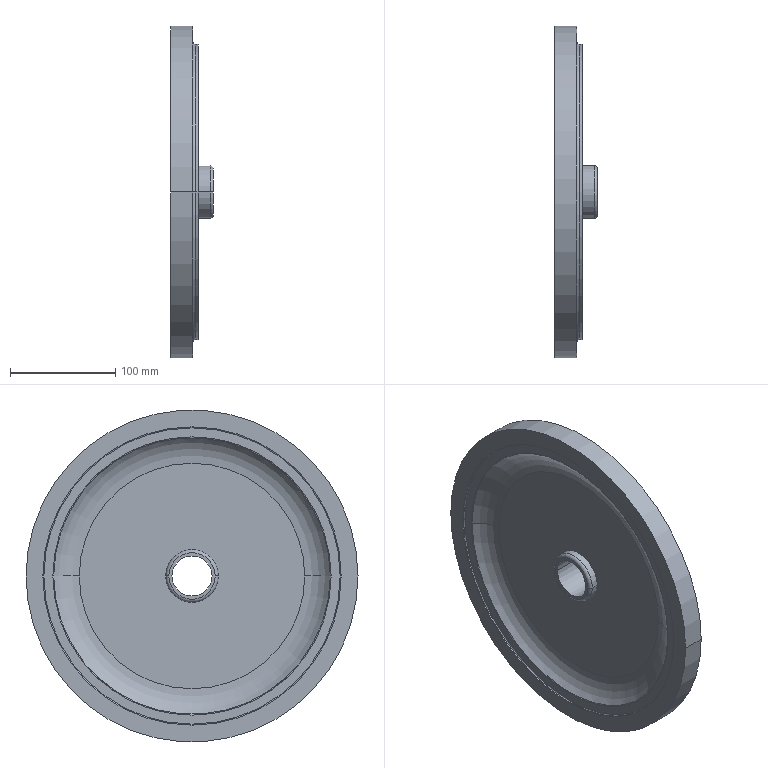Part | SolidWorks | features Revolution 1 | 1 solid | 31 faces | box 40.5 x 315 x 315 mm | volume 1243951 mm3 | torus 12 | cylinder 12 | plane 7 | commonest cylinder face diameters 50 x4 38 x2 280 x2 283 x2 315 x2
STEP:
#1=CARTESIAN_POINT('',(-149.425,-131.204,0.));
#2=VERTEX_POINT('',#1);
#3=CARTESIAN_POINT('',(-149.425,131.204,0.));
#4=VERTEX_POINT('',#3);
#5=CARTESIAN_POINT('',(-149.425,0.,0.));
#6=DIRECTION('',(1.,0.,0.));
#7=DIRECTION('',(0.,1.,0.));
#8=AXIS2_PLACEMENT_3D('',#5,#6,#7);
#9=CIRCLE('',#8,131.204);
#10=EDGE_CURVE('',#2,#4,#9,.T.);
#11=ORIENTED_EDGE('',*,*,#10,.F.);
#12=CARTESIAN_POINT('',(-137.8,-107.,0.));
#13=VERTEX_POINT('',#12);
#14=CARTESIAN_POINT('',(-168.81,-107.,0.));
#15=DIRECTION('',(0.,0.,1.));
#16=DIRECTION('',(0.,-1.,0.));
#17=AXIS2_PLACEMENT_3D('',#14,#15,#16);
#18=CIRCLE('',#17,31.01);
#19=EDGE_CURVE('',#2,#13,#18,.T.);
#20=ORIENTED_EDGE('',*,*,#19,.T.);
#21=CARTESIAN_POINT('',(-137.8,107.,0.));
#22=VERTEX_POINT('',#21);
#23=CARTESIAN_POINT('',(-137.8,0.,0.));
#24=DIRECTION('',(1.,0.,0.));
#25=DIRECTION('',(0.,1.,0.));
#26=AXIS2_PLACEMENT_3D('',#23,#24,#25);
#27=CIRCLE('',#26,107.);
#28=EDGE_CURVE('',#13,#22,#27,.T.);
#29=ORIENTED_EDGE('',*,*,#28,.T.);
#30=CARTESIAN_POINT('',(-168.81,107.,0.));
#31=DIRECTION('',(0.,0.,-1.));
#32=DIRECTION('',(-1.,0.,0.));
#33=AXIS2_PLACEMENT_3D('',#30,#31,#32);
#34=CIRCLE('',#33,31.01);
#35=EDGE_CURVE('',#4,#22,#34,.T.);
#36=ORIENTED_EDGE('',*,*,#35,.F.);
#37=EDGE_LOOP('',(#11,#20,#29,#36));
#38=FACE_OUTER_BOUND('',#37,.T.);
#39=CARTESIAN_POINT('',(-168.81,0.,0.));
#40=DIRECTION('',(1.,0.,0.));
#41=DIRECTION('',(0.,1.,0.));
#42=AXIS2_PLACEMENT_3D('',#39,#40,#41);
#43=TOROIDAL_SURFACE('',#42,107.,31.01);
#44=ADVANCED_FACE('',(#38),#43,.F.);
#45=CARTESIAN_POINT('',(-149.425,0.,0.));
#46=DIRECTION('',(1.,0.,0.));
#47=DIRECTION('',(0.,1.,0.));
#48=AXIS2_PLACEMENT_3D('',#45,#46,#47);
#49=CIRCLE('',#48,131.204);
#50=EDGE_CURVE('',#4,#2,#49,.T.);
#51=ORIENTED_EDGE('',*,*,#50,.T.);
#52=CARTESIAN_POINT('',(-149.8,-131.985,0.));
#53=VERTEX_POINT('',#52);
#54=CARTESIAN_POINT('',(-148.8,-131.985,0.));
#55=DIRECTION('',(0.,0.,1.));
#56=DIRECTION('',(0.,-1.,0.));
#57=AXIS2_PLACEMENT_3D('',#54,#55,#56);
#58=CIRCLE('',#57,1.);
#59=EDGE_CURVE('',#2,#53,#58,.T.);
#60=ORIENTED_EDGE('',*,*,#59,.T.);
#61=CARTESIAN_POINT('',(-149.8,131.985,0.));
#62=VERTEX_POINT('',#61);
#63=CARTESIAN_POINT('',(-149.8,0.,0.));
#64=DIRECTION('',(1.,0.,0.));
#65=DIRECTION('',(0.,1.,0.));
#66=AXIS2_PLACEMENT_3D('',#63,#64,#65);
#67=CIRCLE('',#66,131.985);
#68=EDGE_CURVE('',#62,#53,#67,.T.);
#69=ORIENTED_EDGE('',*,*,#68,.F.);
#70=CARTESIAN_POINT('',(-148.8,131.985,0.));
#71=DIRECTION('',(0.,0.,-1.));
#72=DIRECTION('',(-1.,0.,0.));
#73=AXIS2_PLACEMENT_3D('',#70,#71,#72);
#74=CIRCLE('',#73,1.);
#75=EDGE_CURVE('',#4,#62,#74,.T.);
#76=ORIENTED_EDGE('',*,*,#75,.F.);
#77=EDGE_LOOP('',(#51,#60,#69,#76));
#78=FACE_OUTER_BOUND('',#77,.T.);
#79=CARTESIAN_POINT('',(-148.8,0.,0.));
#80=DIRECTION('',(1.,0.,0.));
#81=DIRECTION('',(0.,1.,0.));
#82=AXIS2_PLACEMENT_3D('',#79,#80,#81);
#83=TOROIDAL_SURFACE('',#82,131.985,1.);
#84=ADVANCED_FACE('',(#78),#83,.T.);
#85=CARTESIAN_POINT('',(-150.8,-141.5,0.));
#86=VERTEX_POINT('',#85);
#87=CARTESIAN_POINT('',(-150.8,141.5,0.));
#88=VERTEX_POINT('',#87);
#89=CARTESIAN_POINT('',(-150.8,0.,0.));
#90=DIRECTION('',(1.,0.,0.));
#91=DIRECTION('',(0.,1.,0.));
#92=AXIS2_PLACEMENT_3D('',#89,#90,#91);
#93=CIRCLE('',#92,141.5);
#94=EDGE_CURVE('',#86,#88,#93,.T.);
#95=ORIENTED_EDGE('',*,*,#94,.F.);
#96=CARTESIAN_POINT('',(-149.8,-140.5,0.));
#97=VERTEX_POINT('',#96);
#98=CARTESIAN_POINT('',(-150.8,-140.5,0.));
#99=DIRECTION('',(0.,0.,1.));
#100=DIRECTION('',(0.,-1.,0.));
#101=AXIS2_PLACEMENT_3D('',#98,#99,#100);
#102=CIRCLE('',#101,1.);
#103=EDGE_CURVE('',#86,#97,#102,.T.);
#104=ORIENTED_EDGE('',*,*,#103,.T.);
#105=CARTESIAN_POINT('',(-149.8,140.5,0.));
#106=VERTEX_POINT('',#105);
#107=CARTESIAN_POINT('',(-149.8,0.,0.));
#108=DIRECTION('',(1.,0.,0.));
#109=DIRECTION('',(0.,1.,0.));
#110=AXIS2_PLACEMENT_3D('',#107,#108,#109);
#111=CIRCLE('',#110,140.5);
#112=EDGE_CURVE('',#97,#106,#111,.T.);
#113=ORIENTED_EDGE('',*,*,#112,.T.);
#114=CARTESIAN_POINT('',(-150.8,140.5,0.));
#115=DIRECTION('',(0.,0.,-1.));
#116=DIRECTION('',(-1.,0.,0.));
#117=AXIS2_PLACEMENT_3D('',#114,#115,#116);
#118=CIRCLE('',#117,1.);
#119=EDGE_CURVE('',#88,#106,#118,.T.);
#120=ORIENTED_EDGE('',*,*,#119,.F.);
#121=EDGE_LOOP('',(#95,#104,#113,#120));
#122=FACE_OUTER_BOUND('',#121,.T.);
#123=CARTESIAN_POINT('',(-150.8,0.,0.));
#124=DIRECTION('',(1.,0.,0.));
#125=DIRECTION('',(0.,1.,0.));
#126=AXIS2_PLACEMENT_3D('',#123,#124,#125);
#127=TOROIDAL_SURFACE('',#126,140.5,1.);
#128=ADVANCED_FACE('',(#122),#127,.F.);
#129=CARTESIAN_POINT('',(-151.8,-141.5,0.));
#130=VERTEX_POINT('',#129);
#131=CARTESIAN_POINT('',(-151.8,141.5,0.));
#132=VERTEX_POINT('',#131);
#133=CARTESIAN_POINT('',(-151.8,0.,0.));
#134=DIRECTION('',(1.,0.,0.));
#135=DIRECTION('',(0.,1.,0.));
#136=AXIS2_PLACEMENT_3D('',#133,#134,#135);
#137=CIRCLE('',#136,141.5);
#138=EDGE_CURVE('',#130,#132,#137,.T.);
#139=ORIENTED_EDGE('',*,*,#138,.F.);
#140=CARTESIAN_POINT('',(-55.,-141.5,0.));
#141=DIRECTION('',(1.,0.,0.));
#142=VECTOR('',#141,1000.);
#143=LINE('',#140,#142);
#144=EDGE_CURVE('',#130,#86,#143,.T.);
#145=ORIENTED_EDGE('',*,*,#144,.T.);
#146=ORIENTED_EDGE('',*,*,#94,.T.);
#147=CARTESIAN_POINT('',(-55.,141.5,0.));
#148=DIRECTION('',(1.,0.,0.));
#149=VECTOR('',#148,1000.);
#150=LINE('',#147,#149);
#151=EDGE_CURVE('',#132,#88,#150,.T.);
#152=ORIENTED_EDGE('',*,*,#151,.F.);
#153=EDGE_LOOP('',(#139,#145,#146,#152));
#154=FACE_OUTER_BOUND('',#153,.T.);
#155=CARTESIAN_POINT('',(-55.,0.,0.));
#156=DIRECTION('',(1.,0.,0.));
#157=DIRECTION('',(0.,1.,0.));
#158=AXIS2_PLACEMENT_3D('',#155,#156,#157);
#159=CYLINDRICAL_SURFACE('',#158,141.5);
#160=ADVANCED_FACE('',(#154),#159,.F.);
#161=CARTESIAN_POINT('',(-151.8,157.5,0.));
#162=VERTEX_POINT('',#161);
#163=CARTESIAN_POINT('',(-151.8,-157.5,0.));
#164=VERTEX_POINT('',#163);
#165=CARTESIAN_POINT('',(-151.8,0.,0.));
#166=DIRECTION('',(1.,0.,0.));
#167=DIRECTION('',(0.,1.,0.));
#168=AXIS2_PLACEMENT_3D('',#165,#166,#167);
#169=CIRCLE('',#168,157.5);
#170=EDGE_CURVE('',#162,#164,#169,.T.);
#171=ORIENTED_EDGE('',*,*,#170,.T.);
#172=CARTESIAN_POINT('',(-130.8,-157.5,0.));
#173=VERTEX_POINT('',#172);
#174=CARTESIAN_POINT('',(-55.,-157.5,0.));
#175=DIRECTION('',(1.,0.,0.));
#176=VECTOR('',#175,1000.);
#177=LINE('',#174,#176);
#178=EDGE_CURVE('',#164,#173,#177,.T.);
#179=ORIENTED_EDGE('',*,*,#178,.T.);
#180=CARTESIAN_POINT('',(-130.8,157.5,0.));
#181=VERTEX_POINT('',#180);
#182=CARTESIAN_POINT('',(-130.8,0.,0.));
#183=DIRECTION('',(1.,0.,0.));
#184=DIRECTION('',(0.,1.,0.));
#185=AXIS2_PLACEMENT_3D('',#182,#183,#184);
#186=CIRCLE('',#185,157.5);
#187=EDGE_CURVE('',#181,#173,#186,.T.);
#188=ORIENTED_EDGE('',*,*,#187,.F.);
#189=CARTESIAN_POINT('',(-55.,157.5,0.));
#190=DIRECTION('',(1.,0.,0.));
#191=VECTOR('',#190,1000.);
#192=LINE('',#189,#191);
#193=EDGE_CURVE('',#162,#181,#192,.T.);
#194=ORIENTED_EDGE('',*,*,#193,.F.);
#195=EDGE_LOOP('',(#171,#179,#188,#194));
#196=FACE_OUTER_BOUND('',#195,.T.);
#197=CARTESIAN_POINT('',(-55.,0.,0.));
#198=DIRECTION('',(1.,0.,0.));
#199=DIRECTION('',(0.,1.,0.));
#200=AXIS2_PLACEMENT_3D('',#197,#198,#199);
#201=CYLINDRICAL_SURFACE('',#200,157.5);
#202=ADVANCED_FACE('',(#196),#201,.T.);
#203=CARTESIAN_POINT('',(-128.3,-140.,0.));
#204=VERTEX_POINT('',#203);
#205=CARTESIAN_POINT('',(-128.3,140.,0.));
#206=VERTEX_POINT('',#205);
#207=CARTESIAN_POINT('',(-128.3,0.,0.));
#208=DIRECTION('',(1.,0.,0.));
#209=DIRECTION('',(0.,1.,0.));
#210=AXIS2_PLACEMENT_3D('',#207,#208,#209);
#211=CIRCLE('',#210,140.);
#212=EDGE_CURVE('',#204,#206,#211,.T.);
#213=ORIENTED_EDGE('',*,*,#212,.F.);
#214=CARTESIAN_POINT('',(-130.8,-142.5,0.));
#215=VERTEX_POINT('',#214);
#216=CARTESIAN_POINT('',(-128.3,-142.5,0.));
#217=DIRECTION('',(0.,0.,1.));
#218=DIRECTION('',(0.,-1.,0.));
#219=AXIS2_PLACEMENT_3D('',#216,#217,#218);
#220=CIRCLE('',#219,2.5);
#221=EDGE_CURVE('',#204,#215,#220,.T.);
#222=ORIENTED_EDGE('',*,*,#221,.T.);
#223=CARTESIAN_POINT('',(-130.8,142.5,0.));
#224=VERTEX_POINT('',#223);
#225=CARTESIAN_POINT('',(-130.8,0.,0.));
#226=DIRECTION('',(1.,0.,0.));
#227=DIRECTION('',(0.,1.,0.));
#228=AXIS2_PLACEMENT_3D('',#225,#226,#227);
#229=CIRCLE('',#228,142.5);
#230=EDGE_CURVE('',#215,#224,#229,.T.);
#231=ORIENTED_EDGE('',*,*,#230,.T.);
#232=CARTESIAN_POINT('',(-128.3,142.5,0.));
#233=DIRECTION('',(0.,0.,-1.));
#234=DIRECTION('',(-1.,0.,0.));
#235=AXIS2_PLACEMENT_3D('',#232,#233,#234);
#236=CIRCLE('',#235,2.5);
#237=EDGE_CURVE('',#206,#224,#236,.T.);
#238=ORIENTED_EDGE('',*,*,#237,.F.);
#239=EDGE_LOOP('',(#213,#222,#231,#238));
#240=FACE_OUTER_BOUND('',#239,.T.);
#241=CARTESIAN_POINT('',(-128.3,0.,0.));
#242=DIRECTION('',(1.,0.,0.));
#243=DIRECTION('',(0.,1.,0.));
#244=AXIS2_PLACEMENT_3D('',#241,#242,#243);
#245=TOROIDAL_SURFACE('',#244,142.5,2.5);
#246=ADVANCED_FACE('',(#240),#245,.F.);
#247=CARTESIAN_POINT('',(-128.3,0.,0.));
#248=DIRECTION('',(1.,0.,0.));
#249=DIRECTION('',(0.,1.,0.));
#250=AXIS2_PLACEMENT_3D('',#247,#248,#249);
#251=CIRCLE('',#250,140.);
#252=EDGE_CURVE('',#206,#204,#251,.T.);
#253=ORIENTED_EDGE('',*,*,#252,.T.);
#254=CARTESIAN_POINT('',(-125.8,-140.,0.));
#255=VERTEX_POINT('',#254);
#256=CARTESIAN_POINT('',(-55.,-140.,0.));
#257=DIRECTION('',(1.,0.,0.));
#258=VECTOR('',#257,1000.);
#259=LINE('',#256,#258);
#260=EDGE_CURVE('',#204,#255,#259,.T.);
#261=ORIENTED_EDGE('',*,*,#260,.T.);
#262=CARTESIAN_POINT('',(-125.8,140.,0.));
#263=VERTEX_POINT('',#262);
#264=CARTESIAN_POINT('',(-125.8,0.,0.));
#265=DIRECTION('',(1.,0.,0.));
#266=DIRECTION('',(0.,1.,0.));
#267=AXIS2_PLACEMENT_3D('',#264,#265,#266);
#268=CIRCLE('',#267,140.);
#269=EDGE_CURVE('',#263,#255,#268,.T.);
#270=ORIENTED_EDGE('',*,*,#269,.F.);
#271=CARTESIAN_POINT('',(-55.,140.,0.));
#272=DIRECTION('',(1.,0.,0.));
#273=VECTOR('',#272,1000.);
#274=LINE('',#271,#273);
#275=EDGE_CURVE('',#206,#263,#274,.T.);
#276=ORIENTED_EDGE('',*,*,#275,.F.);
#277=EDGE_LOOP('',(#253,#261,#270,#276));
#278=FACE_OUTER_BOUND('',#277,.T.);
#279=CARTESIAN_POINT('',(-55.,0.,0.));
#280=DIRECTION('',(1.,0.,0.));
#281=DIRECTION('',(0.,1.,0.));
#282=AXIS2_PLACEMENT_3D('',#279,#280,#281);
#283=CYLINDRICAL_SURFACE('',#282,140.);
#284=ADVANCED_FACE('',(#278),#283,.T.);
#285=CARTESIAN_POINT('',(-125.8,25.,0.));
#286=VERTEX_POINT('',#285);
#287=CARTESIAN_POINT('',(-125.8,-25.,0.));
#288=VERTEX_POINT('',#287);
#289=CARTESIAN_POINT('',(-125.8,0.,0.));
#290=DIRECTION('',(1.,0.,0.));
#291=DIRECTION('',(0.,1.,0.));
#292=AXIS2_PLACEMENT_3D('',#289,#290,#291);
#293=CIRCLE('',#292,25.);
#294=EDGE_CURVE('',#286,#288,#293,.T.);
#295=ORIENTED_EDGE('',*,*,#294,.T.);
#296=CARTESIAN_POINT('',(-114.3,-25.,0.));
#297=VERTEX_POINT('',#296);
#298=CARTESIAN_POINT('',(-55.,-25.,0.));
#299=DIRECTION('',(1.,0.,0.));
#300=VECTOR('',#299,1000.);
#301=LINE('',#298,#300);
#302=EDGE_CURVE('',#288,#297,#301,.T.);
#303=ORIENTED_EDGE('',*,*,#302,.T.);
#304=CARTESIAN_POINT('',(-114.3,25.,0.));
#305=VERTEX_POINT('',#304);
#306=CARTESIAN_POINT('',(-114.3,0.,0.));
#307=DIRECTION('',(1.,0.,0.));
#308=DIRECTION('',(0.,1.,0.));
#309=AXIS2_PLACEMENT_3D('',#306,#307,#308);
#310=CIRCLE('',#309,25.);
#311=EDGE_CURVE('',#305,#297,#310,.T.);
#312=ORIENTED_EDGE('',*,*,#311,.F.);
#313=CARTESIAN_POINT('',(-55.,25.,0.));
#314=DIRECTION('',(1.,0.,0.));
#315=VECTOR('',#314,1000.);
#316=LINE('',#313,#315);
#317=EDGE_CURVE('',#286,#305,#316,.T.);
#318=ORIENTED_EDGE('',*,*,#317,.F.);
#319=EDGE_LOOP('',(#295,#303,#312,#318));
#320=FACE_OUTER_BOUND('',#319,.T.);
#321=CARTESIAN_POINT('',(-55.,0.,0.));
#322=DIRECTION('',(1.,0.,0.));
#323=DIRECTION('',(0.,1.,0.));
#324=AXIS2_PLACEMENT_3D('',#321,#322,#323);
#325=CYLINDRICAL_SURFACE('',#324,25.);
#326=ADVANCED_FACE('',(#320),#325,.T.);
#327=ORIENTED_EDGE('',*,*,#311,.T.);
#328=CARTESIAN_POINT('',(-111.3,-22.,0.));
#329=VERTEX_POINT('',#328);
#330=CARTESIAN_POINT('',(-114.3,-22.,0.));
#331=DIRECTION('',(0.,0.,1.));
#332=DIRECTION('',(0.,-1.,0.));
#333=AXIS2_PLACEMENT_3D('',#330,#331,#332);
#334=CIRCLE('',#333,3.);
#335=EDGE_CURVE('',#297,#329,#334,.T.);
#336=ORIENTED_EDGE('',*,*,#335,.T.);
#337=CARTESIAN_POINT('',(-111.3,22.,0.));
#338=VERTEX_POINT('',#337);
#339=CARTESIAN_POINT('',(-111.3,0.,0.));
#340=DIRECTION('',(1.,0.,0.));
#341=DIRECTION('',(0.,1.,0.));
#342=AXIS2_PLACEMENT_3D('',#339,#340,#341);
#343=CIRCLE('',#342,22.);
#344=EDGE_CURVE('',#338,#329,#343,.T.);
#345=ORIENTED_EDGE('',*,*,#344,.F.);
#346=CARTESIAN_POINT('',(-114.3,22.,0.));
#347=DIRECTION('',(0.,0.,-1.));
#348=DIRECTION('',(-1.,0.,0.));
#349=AXIS2_PLACEMENT_3D('',#346,#347,#348);
#350=CIRCLE('',#349,3.);
#351=EDGE_CURVE('',#305,#338,#350,.T.);
#352=ORIENTED_EDGE('',*,*,#351,.F.);
#353=EDGE_LOOP('',(#327,#336,#345,#352));
#354=FACE_OUTER_BOUND('',#353,.T.);
#355=CARTESIAN_POINT('',(-114.3,0.,0.));
#356=DIRECTION('',(1.,0.,0.));
#357=DIRECTION('',(0.,1.,0.));
#358=AXIS2_PLACEMENT_3D('',#355,#356,#357);
#359=TOROIDAL_SURFACE('',#358,22.,3.);
#360=ADVANCED_FACE('',(#354),#359,.T.);
#361=CARTESIAN_POINT('',(-147.3,-19.,0.));
#362=VERTEX_POINT('',#361);
#363=CARTESIAN_POINT('',(-147.3,19.,0.));
#364=VERTEX_POINT('',#363);
#365=CARTESIAN_POINT('',(-147.3,0.,0.));
#366=DIRECTION('',(1.,0.,0.));
#367=DIRECTION('',(0.,1.,0.));
#368=AXIS2_PLACEMENT_3D('',#365,#366,#367);
#369=CIRCLE('',#368,19.);
#370=EDGE_CURVE('',#362,#364,#369,.T.);
#371=ORIENTED_EDGE('',*,*,#370,.F.);
#372=CARTESIAN_POINT('',(-111.3,-19.,0.));
#373=VERTEX_POINT('',#372);
#374=CARTESIAN_POINT('',(-55.,-19.,0.));
#375=DIRECTION('',(1.,0.,0.));
#376=VECTOR('',#375,1000.);
#377=LINE('',#374,#376);
#378=EDGE_CURVE('',#362,#373,#377,.T.);
#379=ORIENTED_EDGE('',*,*,#378,.T.);
#380=CARTESIAN_POINT('',(-111.3,19.,0.));
#381=VERTEX_POINT('',#380);
#382=CARTESIAN_POINT('',(-111.3,0.,0.));
#383=DIRECTION('',(1.,0.,0.));
#384=DIRECTION('',(0.,1.,0.));
#385=AXIS2_PLACEMENT_3D('',#382,#383,#384);
#386=CIRCLE('',#385,19.);
#387=EDGE_CURVE('',#373,#381,#386,.T.);
#388=ORIENTED_EDGE('',*,*,#387,.T.);
#389=CARTESIAN_POINT('',(-55.,19.,0.));
#390=DIRECTION('',(1.,0.,0.));
#391=VECTOR('',#390,1000.);
#392=LINE('',#389,#391);
#393=EDGE_CURVE('',#364,#381,#392,.T.);
#394=ORIENTED_EDGE('',*,*,#393,.F.);
#395=EDGE_LOOP('',(#371,#379,#388,#394));
#396=FACE_OUTER_BOUND('',#395,.T.);
#397=CARTESIAN_POINT('',(-55.,0.,0.));
#398=DIRECTION('',(1.,0.,0.));
#399=DIRECTION('',(0.,1.,0.));
#400=AXIS2_PLACEMENT_3D('',#397,#398,#399);
#401=CYLINDRICAL_SURFACE('',#400,19.);
#402=ADVANCED_FACE('',(#396),#401,.F.);
#403=CARTESIAN_POINT('',(-147.3,22.,0.));
#404=VERTEX_POINT('',#403);
#405=CARTESIAN_POINT('',(-147.3,-22.,0.));
#406=VERTEX_POINT('',#405);
#407=CARTESIAN_POINT('',(-147.3,0.,0.));
#408=DIRECTION('',(1.,0.,0.));
#409=DIRECTION('',(0.,1.,0.));
#410=AXIS2_PLACEMENT_3D('',#407,#408,#409);
#411=CIRCLE('',#410,22.);
#412=EDGE_CURVE('',#404,#406,#411,.T.);
#413=ORIENTED_EDGE('',*,*,#412,.T.);
#414=CARTESIAN_POINT('',(-144.3,-25.,0.));
#415=VERTEX_POINT('',#414);
#416=CARTESIAN_POINT('',(-144.3,-22.,0.));
#417=DIRECTION('',(0.,0.,1.));
#418=DIRECTION('',(0.,-1.,0.));
#419=AXIS2_PLACEMENT_3D('',#416,#417,#418);
#420=CIRCLE('',#419,3.);
#421=EDGE_CURVE('',#406,#415,#420,.T.);
#422=ORIENTED_EDGE('',*,*,#421,.T.);
#423=CARTESIAN_POINT('',(-144.3,25.,0.));
#424=VERTEX_POINT('',#423);
#425=CARTESIAN_POINT('',(-144.3,0.,0.));
#426=DIRECTION('',(1.,0.,0.));
#427=DIRECTION('',(0.,1.,0.));
#428=AXIS2_PLACEMENT_3D('',#425,#426,#427);
#429=CIRCLE('',#428,25.);
#430=EDGE_CURVE('',#424,#415,#429,.T.);
#431=ORIENTED_EDGE('',*,*,#430,.F.);
#432=CARTESIAN_POINT('',(-144.3,22.,0.));
#433=DIRECTION('',(0.,0.,-1.));
#434=DIRECTION('',(-1.,0.,0.));
#435=AXIS2_PLACEMENT_3D('',#432,#433,#434);
#436=CIRCLE('',#435,3.);
#437=EDGE_CURVE('',#404,#424,#436,.T.);
#438=ORIENTED_EDGE('',*,*,#437,.F.);
#439=EDGE_LOOP('',(#413,#422,#431,#438));
#440=FACE_OUTER_BOUND('',#439,.T.);
#441=CARTESIAN_POINT('',(-144.3,0.,0.));
#442=DIRECTION('',(1.,0.,0.));
#443=DIRECTION('',(0.,1.,0.));
#444=AXIS2_PLACEMENT_3D('',#441,#442,#443);
#445=TOROIDAL_SURFACE('',#444,22.,3.);
#446=ADVANCED_FACE('',(#440),#445,.T.);
#447=ORIENTED_EDGE('',*,*,#430,.T.);
#448=CARTESIAN_POINT('',(-137.8,-25.,0.));
#449=VERTEX_POINT('',#448);
#450=CARTESIAN_POINT('',(-55.,-25.,0.));
#451=DIRECTION('',(1.,0.,0.));
#452=VECTOR('',#451,1000.);
#453=LINE('',#450,#452);
#454=EDGE_CURVE('',#415,#449,#453,.T.);
#455=ORIENTED_EDGE('',*,*,#454,.T.);
#456=CARTESIAN_POINT('',(-137.8,25.,0.));
#457=VERTEX_POINT('',#456);
#458=CARTESIAN_POINT('',(-137.8,0.,0.));
#459=DIRECTION('',(1.,0.,0.));
#460=DIRECTION('',(0.,1.,0.));
#461=AXIS2_PLACEMENT_3D('',#458,#459,#460);
#462=CIRCLE('',#461,25.);
#463=EDGE_CURVE('',#457,#449,#462,.T.);
#464=ORIENTED_EDGE('',*,*,#463,.F.);
#465=CARTESIAN_POINT('',(-55.,25.,0.));
#466=DIRECTION('',(1.,0.,0.));
#467=VECTOR('',#466,1000.);
#468=LINE('',#465,#467);
#469=EDGE_CURVE('',#424,#457,#468,.T.);
#470=ORIENTED_EDGE('',*,*,#469,.F.);
#471=EDGE_LOOP('',(#447,#455,#464,#470));
#472=FACE_OUTER_BOUND('',#471,.T.);
#473=CARTESIAN_POINT('',(-55.,0.,0.));
#474=DIRECTION('',(1.,0.,0.));
#475=DIRECTION('',(0.,1.,0.));
#476=AXIS2_PLACEMENT_3D('',#473,#474,#475);
#477=CYLINDRICAL_SURFACE('',#476,25.);
#478=ADVANCED_FACE('',(#472),#477,.T.);
#479=ORIENTED_EDGE('',*,*,#454,.F.);
#480=CARTESIAN_POINT('',(-144.3,0.,0.));
#481=DIRECTION('',(1.,0.,0.));
#482=DIRECTION('',(0.,1.,0.));
#483=AXIS2_PLACEMENT_3D('',#480,#481,#482);
#484=CIRCLE('',#483,25.);
#485=EDGE_CURVE('',#415,#424,#484,.T.);
#486=ORIENTED_EDGE('',*,*,#485,.T.);
#487=ORIENTED_EDGE('',*,*,#469,.T.);
#488=CARTESIAN_POINT('',(-137.8,0.,0.));
#489=DIRECTION('',(1.,0.,0.));
#490=DIRECTION('',(0.,1.,0.));
#491=AXIS2_PLACEMENT_3D('',#488,#489,#490);
#492=CIRCLE('',#491,25.);
#493=EDGE_CURVE('',#449,#457,#492,.T.);
#494=ORIENTED_EDGE('',*,*,#493,.F.);
#495=EDGE_LOOP('',(#479,#486,#487,#494));
#496=FACE_OUTER_BOUND('',#495,.T.);
#497=CARTESIAN_POINT('',(-55.,0.,0.));
#498=DIRECTION('',(1.,0.,0.));
#499=DIRECTION('',(0.,1.,0.));
#500=AXIS2_PLACEMENT_3D('',#497,#498,#499);
#501=CYLINDRICAL_SURFACE('',#500,25.);
#502=ADVANCED_FACE('',(#496),#501,.T.);
#503=ORIENTED_EDGE('',*,*,#421,.F.);
#504=CARTESIAN_POINT('',(-147.3,0.,0.));
#505=DIRECTION('',(1.,0.,0.));
#506=DIRECTION('',(0.,1.,0.));
#507=AXIS2_PLACEMENT_3D('',#504,#505,#506);
#508=CIRCLE('',#507,22.);
#509=EDGE_CURVE('',#406,#404,#508,.T.);
#510=ORIENTED_EDGE('',*,*,#509,.T.);
#511=ORIENTED_EDGE('',*,*,#437,.T.);
#512=ORIENTED_EDGE('',*,*,#485,.F.);
#513=EDGE_LOOP('',(#503,#510,#511,#512));
#514=FACE_OUTER_BOUND('',#513,.T.);
#515=CARTESIAN_POINT('',(-144.3,0.,0.));
#516=DIRECTION('',(1.,0.,0.));
#517=DIRECTION('',(0.,1.,0.));
#518=AXIS2_PLACEMENT_3D('',#515,#516,#517);
#519=TOROIDAL_SURFACE('',#518,22.,3.);
#520=ADVANCED_FACE('',(#514),#519,.T.);
#521=CARTESIAN_POINT('',(-147.3,0.,0.));
#522=DIRECTION('',(1.,0.,0.));
#523=DIRECTION('',(0.,1.,0.));
#524=AXIS2_PLACEMENT_3D('',#521,#522,#523);
#525=CIRCLE('',#524,19.);
#526=EDGE_CURVE('',#364,#362,#525,.T.);
#527=ORIENTED_EDGE('',*,*,#526,.T.);
#528=ORIENTED_EDGE('',*,*,#370,.T.);
#529=EDGE_LOOP('',(#527,#528));
#530=FACE_BOUND('',#529,.T.);
#531=ORIENTED_EDGE('',*,*,#412,.F.);
#532=ORIENTED_EDGE('',*,*,#509,.F.);
#533=EDGE_LOOP('',(#531,#532));
#534=FACE_OUTER_BOUND('',#533,.T.);
#535=CARTESIAN_POINT('',(-147.3,22.,0.));
#536=DIRECTION('',(-1.,0.,0.));
#537=DIRECTION('',(0.,-1.,0.));
#538=AXIS2_PLACEMENT_3D('',#535,#536,#537);
#539=PLANE('',#538);
#540=ADVANCED_FACE('',(#530,#534),#539,.T.);
#541=ORIENTED_EDGE('',*,*,#378,.F.);
#542=ORIENTED_EDGE('',*,*,#526,.F.);
#543=ORIENTED_EDGE('',*,*,#393,.T.);
#544=CARTESIAN_POINT('',(-111.3,0.,0.));
#545=DIRECTION('',(1.,0.,0.));
#546=DIRECTION('',(0.,1.,0.));
#547=AXIS2_PLACEMENT_3D('',#544,#545,#546);
#548=CIRCLE('',#547,19.);
#549=EDGE_CURVE('',#381,#373,#548,.T.);
#550=ORIENTED_EDGE('',*,*,#549,.T.);
#551=EDGE_LOOP('',(#541,#542,#543,#550));
#552=FACE_OUTER_BOUND('',#551,.T.);
#553=CARTESIAN_POINT('',(-55.,0.,0.));
#554=DIRECTION('',(1.,0.,0.));
#555=DIRECTION('',(0.,1.,0.));
#556=AXIS2_PLACEMENT_3D('',#553,#554,#555);
#557=CYLINDRICAL_SURFACE('',#556,19.);
#558=ADVANCED_FACE('',(#552),#557,.F.);
#559=ORIENTED_EDGE('',*,*,#344,.T.);
#560=CARTESIAN_POINT('',(-111.3,0.,0.));
#561=DIRECTION('',(1.,0.,0.));
#562=DIRECTION('',(0.,1.,0.));
#563=AXIS2_PLACEMENT_3D('',#560,#561,#562);
#564=CIRCLE('',#563,22.);
#565=EDGE_CURVE('',#329,#338,#564,.T.);
#566=ORIENTED_EDGE('',*,*,#565,.T.);
#567=EDGE_LOOP('',(#559,#566));
#568=FACE_OUTER_BOUND('',#567,.T.);
#569=ORIENTED_EDGE('',*,*,#549,.F.);
#570=ORIENTED_EDGE('',*,*,#387,.F.);
#571=EDGE_LOOP('',(#569,#570));
#572=FACE_BOUND('',#571,.T.);
#573=CARTESIAN_POINT('',(-111.3,22.,0.));
#574=DIRECTION('',(1.,0.,0.));
#575=DIRECTION('',(0.,1.,0.));
#576=AXIS2_PLACEMENT_3D('',#573,#574,#575);
#577=PLANE('',#576);
#578=ADVANCED_FACE('',(#568,#572),#577,.T.);
#579=ORIENTED_EDGE('',*,*,#335,.F.);
#580=CARTESIAN_POINT('',(-114.3,0.,0.));
#581=DIRECTION('',(1.,0.,0.));
#582=DIRECTION('',(0.,1.,0.));
#583=AXIS2_PLACEMENT_3D('',#580,#581,#582);
#584=CIRCLE('',#583,25.);
#585=EDGE_CURVE('',#297,#305,#584,.T.);
#586=ORIENTED_EDGE('',*,*,#585,.T.);
#587=ORIENTED_EDGE('',*,*,#351,.T.);
#588=ORIENTED_EDGE('',*,*,#565,.F.);
#589=EDGE_LOOP('',(#579,#586,#587,#588));
#590=FACE_OUTER_BOUND('',#589,.T.);
#591=CARTESIAN_POINT('',(-114.3,0.,0.));
#592=DIRECTION('',(1.,0.,0.));
#593=DIRECTION('',(0.,1.,0.));
#594=AXIS2_PLACEMENT_3D('',#591,#592,#593);
#595=TOROIDAL_SURFACE('',#594,22.,3.);
#596=ADVANCED_FACE('',(#590),#595,.T.);
#597=ORIENTED_EDGE('',*,*,#302,.F.);
#598=CARTESIAN_POINT('',(-125.8,0.,0.));
#599=DIRECTION('',(1.,0.,0.));
#600=DIRECTION('',(0.,1.,0.));
#601=AXIS2_PLACEMENT_3D('',#598,#599,#600);
#602=CIRCLE('',#601,25.);
#603=EDGE_CURVE('',#288,#286,#602,.T.);
#604=ORIENTED_EDGE('',*,*,#603,.T.);
#605=ORIENTED_EDGE('',*,*,#317,.T.);
#606=ORIENTED_EDGE('',*,*,#585,.F.);
#607=EDGE_LOOP('',(#597,#604,#605,#606));
#608=FACE_OUTER_BOUND('',#607,.T.);
#609=CARTESIAN_POINT('',(-55.,0.,0.));
#610=DIRECTION('',(1.,0.,0.));
#611=DIRECTION('',(0.,1.,0.));
#612=AXIS2_PLACEMENT_3D('',#609,#610,#611);
#613=CYLINDRICAL_SURFACE('',#612,25.);
#614=ADVANCED_FACE('',(#608),#613,.T.);
#615=ORIENTED_EDGE('',*,*,#269,.T.);
#616=CARTESIAN_POINT('',(-125.8,0.,0.));
#617=DIRECTION('',(1.,0.,0.));
#618=DIRECTION('',(0.,1.,0.));
#619=AXIS2_PLACEMENT_3D('',#616,#617,#618);
#620=CIRCLE('',#619,140.);
#621=EDGE_CURVE('',#255,#263,#620,.T.);
#622=ORIENTED_EDGE('',*,*,#621,.T.);
#623=EDGE_LOOP('',(#615,#622));
#624=FACE_OUTER_BOUND('',#623,.T.);
#625=ORIENTED_EDGE('',*,*,#294,.F.);
#626=ORIENTED_EDGE('',*,*,#603,.F.);
#627=EDGE_LOOP('',(#625,#626));
#628=FACE_BOUND('',#627,.T.);
#629=CARTESIAN_POINT('',(-125.8,140.,0.));
#630=DIRECTION('',(1.,0.,0.));
#631=DIRECTION('',(0.,1.,0.));
#632=AXIS2_PLACEMENT_3D('',#629,#630,#631);
#633=PLANE('',#632);
#634=ADVANCED_FACE('',(#624,#628),#633,.T.);
#635=ORIENTED_EDGE('',*,*,#260,.F.);
#636=ORIENTED_EDGE('',*,*,#212,.T.);
#637=ORIENTED_EDGE('',*,*,#275,.T.);
#638=ORIENTED_EDGE('',*,*,#621,.F.);
#639=EDGE_LOOP('',(#635,#636,#637,#638));
#640=FACE_OUTER_BOUND('',#639,.T.);
#641=CARTESIAN_POINT('',(-55.,0.,0.));
#642=DIRECTION('',(1.,0.,0.));
#643=DIRECTION('',(0.,1.,0.));
#644=AXIS2_PLACEMENT_3D('',#641,#642,#643);
#645=CYLINDRICAL_SURFACE('',#644,140.);
#646=ADVANCED_FACE('',(#640),#645,.T.);
#647=ORIENTED_EDGE('',*,*,#221,.F.);
#648=ORIENTED_EDGE('',*,*,#252,.F.);
#649=ORIENTED_EDGE('',*,*,#237,.T.);
#650=CARTESIAN_POINT('',(-130.8,0.,0.));
#651=DIRECTION('',(1.,0.,0.));
#652=DIRECTION('',(0.,1.,0.));
#653=AXIS2_PLACEMENT_3D('',#650,#651,#652);
#654=CIRCLE('',#653,142.5);
#655=EDGE_CURVE('',#224,#215,#654,.T.);
#656=ORIENTED_EDGE('',*,*,#655,.T.);
#657=EDGE_LOOP('',(#647,#648,#649,#656));
#658=FACE_OUTER_BOUND('',#657,.T.);
#659=CARTESIAN_POINT('',(-128.3,0.,0.));
#660=DIRECTION('',(1.,0.,0.));
#661=DIRECTION('',(0.,1.,0.));
#662=AXIS2_PLACEMENT_3D('',#659,#660,#661);
#663=TOROIDAL_SURFACE('',#662,142.5,2.5);
#664=ADVANCED_FACE('',(#658),#663,.F.);
#665=ORIENTED_EDGE('',*,*,#187,.T.);
#666=CARTESIAN_POINT('',(-130.8,0.,0.));
#667=DIRECTION('',(1.,0.,0.));
#668=DIRECTION('',(0.,1.,0.));
#669=AXIS2_PLACEMENT_3D('',#666,#667,#668);
#670=CIRCLE('',#669,157.5);
#671=EDGE_CURVE('',#173,#181,#670,.T.);
#672=ORIENTED_EDGE('',*,*,#671,.T.);
#673=EDGE_LOOP('',(#665,#672));
#674=FACE_OUTER_BOUND('',#673,.T.);
#675=ORIENTED_EDGE('',*,*,#655,.F.);
#676=ORIENTED_EDGE('',*,*,#230,.F.);
#677=EDGE_LOOP('',(#675,#676));
#678=FACE_BOUND('',#677,.T.);
#679=CARTESIAN_POINT('',(-130.8,157.5,0.));
#680=DIRECTION('',(1.,0.,0.));
#681=DIRECTION('',(0.,1.,0.));
#682=AXIS2_PLACEMENT_3D('',#679,#680,#681);
#683=PLANE('',#682);
#684=ADVANCED_FACE('',(#674,#678),#683,.T.);
#685=ORIENTED_EDGE('',*,*,#178,.F.);
#686=CARTESIAN_POINT('',(-151.8,0.,0.));
#687=DIRECTION('',(1.,0.,0.));
#688=DIRECTION('',(0.,1.,0.));
#689=AXIS2_PLACEMENT_3D('',#686,#687,#688);
#690=CIRCLE('',#689,157.5);
#691=EDGE_CURVE('',#164,#162,#690,.T.);
#692=ORIENTED_EDGE('',*,*,#691,.T.);
#693=ORIENTED_EDGE('',*,*,#193,.T.);
#694=ORIENTED_EDGE('',*,*,#671,.F.);
#695=EDGE_LOOP('',(#685,#692,#693,#694));
#696=FACE_OUTER_BOUND('',#695,.T.);
#697=CARTESIAN_POINT('',(-55.,0.,0.));
#698=DIRECTION('',(1.,0.,0.));
#699=DIRECTION('',(0.,1.,0.));
#700=AXIS2_PLACEMENT_3D('',#697,#698,#699);
#701=CYLINDRICAL_SURFACE('',#700,157.5);
#702=ADVANCED_FACE('',(#696),#701,.T.);
#703=CARTESIAN_POINT('',(-151.8,0.,0.));
#704=DIRECTION('',(1.,0.,0.));
#705=DIRECTION('',(0.,1.,0.));
#706=AXIS2_PLACEMENT_3D('',#703,#704,#705);
#707=CIRCLE('',#706,141.5);
#708=EDGE_CURVE('',#132,#130,#707,.T.);
#709=ORIENTED_EDGE('',*,*,#708,.T.);
#710=ORIENTED_EDGE('',*,*,#138,.T.);
#711=EDGE_LOOP('',(#709,#710));
#712=FACE_BOUND('',#711,.T.);
#713=ORIENTED_EDGE('',*,*,#170,.F.);
#714=ORIENTED_EDGE('',*,*,#691,.F.);
#715=EDGE_LOOP('',(#713,#714));
#716=FACE_OUTER_BOUND('',#715,.T.);
#717=CARTESIAN_POINT('',(-151.8,145.5,0.));
#718=DIRECTION('',(-1.,0.,0.));
#719=DIRECTION('',(0.,-1.,0.));
#720=AXIS2_PLACEMENT_3D('',#717,#718,#719);
#721=PLANE('',#720);
#722=ADVANCED_FACE('',(#712,#716),#721,.T.);
#723=ORIENTED_EDGE('',*,*,#144,.F.);
#724=ORIENTED_EDGE('',*,*,#708,.F.);
#725=ORIENTED_EDGE('',*,*,#151,.T.);
#726=CARTESIAN_POINT('',(-150.8,0.,0.));
#727=DIRECTION('',(1.,0.,0.));
#728=DIRECTION('',(0.,1.,0.));
#729=AXIS2_PLACEMENT_3D('',#726,#727,#728);
#730=CIRCLE('',#729,141.5);
#731=EDGE_CURVE('',#88,#86,#730,.T.);
#732=ORIENTED_EDGE('',*,*,#731,.T.);
#733=EDGE_LOOP('',(#723,#724,#725,#732));
#734=FACE_OUTER_BOUND('',#733,.T.);
#735=CARTESIAN_POINT('',(-55.,0.,0.));
#736=DIRECTION('',(1.,0.,0.));
#737=DIRECTION('',(0.,1.,0.));
#738=AXIS2_PLACEMENT_3D('',#735,#736,#737);
#739=CYLINDRICAL_SURFACE('',#738,141.5);
#740=ADVANCED_FACE('',(#734),#739,.F.);
#741=ORIENTED_EDGE('',*,*,#103,.F.);
#742=ORIENTED_EDGE('',*,*,#731,.F.);
#743=ORIENTED_EDGE('',*,*,#119,.T.);
#744=CARTESIAN_POINT('',(-149.8,0.,0.));
#745=DIRECTION('',(1.,0.,0.));
#746=DIRECTION('',(0.,1.,0.));
#747=AXIS2_PLACEMENT_3D('',#744,#745,#746);
#748=CIRCLE('',#747,140.5);
#749=EDGE_CURVE('',#106,#97,#748,.T.);
#750=ORIENTED_EDGE('',*,*,#749,.T.);
#751=EDGE_LOOP('',(#741,#742,#743,#750));
#752=FACE_OUTER_BOUND('',#751,.T.);
#753=CARTESIAN_POINT('',(-150.8,0.,0.));
#754=DIRECTION('',(1.,0.,0.));
#755=DIRECTION('',(0.,1.,0.));
#756=AXIS2_PLACEMENT_3D('',#753,#754,#755);
#757=TOROIDAL_SURFACE('',#756,140.5,1.);
#758=ADVANCED_FACE('',(#752),#757,.F.);
#759=ORIENTED_EDGE('',*,*,#68,.T.);
#760=CARTESIAN_POINT('',(-149.8,0.,0.));
#761=DIRECTION('',(1.,0.,0.));
#762=DIRECTION('',(0.,1.,0.));
#763=AXIS2_PLACEMENT_3D('',#760,#761,#762);
#764=CIRCLE('',#763,131.985);
#765=EDGE_CURVE('',#53,#62,#764,.T.);
#766=ORIENTED_EDGE('',*,*,#765,.T.);
#767=EDGE_LOOP('',(#759,#766));
#768=FACE_BOUND('',#767,.T.);
#769=ORIENTED_EDGE('',*,*,#749,.F.);
#770=ORIENTED_EDGE('',*,*,#112,.F.);
#771=EDGE_LOOP('',(#769,#770));
#772=FACE_OUTER_BOUND('',#771,.T.);
#773=CARTESIAN_POINT('',(-149.8,140.5,0.));
#774=DIRECTION('',(-1.,0.,0.));
#775=DIRECTION('',(0.,-1.,0.));
#776=AXIS2_PLACEMENT_3D('',#773,#774,#775);
#777=PLANE('',#776);
#778=ADVANCED_FACE('',(#768,#772),#777,.T.);
#779=ORIENTED_EDGE('',*,*,#59,.F.);
#780=ORIENTED_EDGE('',*,*,#10,.T.);
#781=ORIENTED_EDGE('',*,*,#75,.T.);
#782=ORIENTED_EDGE('',*,*,#765,.F.);
#783=EDGE_LOOP('',(#779,#780,#781,#782));
#784=FACE_OUTER_BOUND('',#783,.T.);
#785=CARTESIAN_POINT('',(-148.8,0.,0.));
#786=DIRECTION('',(1.,0.,0.));
#787=DIRECTION('',(0.,1.,0.));
#788=AXIS2_PLACEMENT_3D('',#785,#786,#787);
#789=TOROIDAL_SURFACE('',#788,131.985,1.);
#790=ADVANCED_FACE('',(#784),#789,.T.);
#791=ORIENTED_EDGE('',*,*,#19,.F.);
#792=ORIENTED_EDGE('',*,*,#50,.F.);
#793=ORIENTED_EDGE('',*,*,#35,.T.);
#794=CARTESIAN_POINT('',(-137.8,0.,0.));
#795=DIRECTION('',(1.,0.,0.));
#796=DIRECTION('',(0.,1.,0.));
#797=AXIS2_PLACEMENT_3D('',#794,#795,#796);
#798=CIRCLE('',#797,107.);
#799=EDGE_CURVE('',#22,#13,#798,.T.);
#800=ORIENTED_EDGE('',*,*,#799,.T.);
#801=EDGE_LOOP('',(#791,#792,#793,#800));
#802=FACE_OUTER_BOUND('',#801,.T.);
#803=CARTESIAN_POINT('',(-168.81,0.,0.));
#804=DIRECTION('',(1.,0.,0.));
#805=DIRECTION('',(0.,1.,0.));
#806=AXIS2_PLACEMENT_3D('',#803,#804,#805);
#807=TOROIDAL_SURFACE('',#806,107.,31.01);
#808=ADVANCED_FACE('',(#802),#807,.F.);
#809=ORIENTED_EDGE('',*,*,#463,.T.);
#810=ORIENTED_EDGE('',*,*,#493,.T.);
#811=EDGE_LOOP('',(#809,#810));
#812=FACE_BOUND('',#811,.T.);
#813=ORIENTED_EDGE('',*,*,#799,.F.);
#814=ORIENTED_EDGE('',*,*,#28,.F.);
#815=EDGE_LOOP('',(#813,#814));
#816=FACE_OUTER_BOUND('',#815,.T.);
#817=CARTESIAN_POINT('',(-137.8,107.,0.));
#818=DIRECTION('',(-1.,0.,0.));
#819=DIRECTION('',(0.,-1.,0.));
#820=AXIS2_PLACEMENT_3D('',#817,#818,#819);
#821=PLANE('',#820);
#822=ADVANCED_FACE('',(#812,#816),#821,.T.);
#823=CLOSED_SHELL('',(#44,#84,#128,#160,#202,#246,#284,#326,#360,#402,#446,#478,#502,#520,#540,#558,#578,#596,#614,#634,#646,#664,#684,#702,#722,#740,#758,#778,#790,#808,#822));
#824=MANIFOLD_SOLID_BREP('',#823);
#825=CARTESIAN_POINT('',(0.,0.,0.));
#826=DIRECTION('',(0.,0.,1.));
#827=DIRECTION('',(1.,0.,0.));
#828=AXIS2_PLACEMENT_3D('',#825,#826,#827);
#829=(LENGTH_UNIT()NAMED_UNIT(*)SI_UNIT(.MILLI.,.METRE.));
#830=UNCERTAINTY_MEASURE_WITH_UNIT(LENGTH_MEASURE(0.00001),#829,'','');
#831=(NAMED_UNIT(*)PLANE_ANGLE_UNIT()SI_UNIT($,.RADIAN.));
#832=(NAMED_UNIT(*)SI_UNIT($,.STERADIAN.)SOLID_ANGLE_UNIT());
#833=(GEOMETRIC_REPRESENTATION_CONTEXT(3)GLOBAL_UNCERTAINTY_ASSIGNED_CONTEXT((#830))GLOBAL_UNIT_ASSIGNED_CONTEXT((#829,#831,#832))REPRESENTATION_CONTEXT('',''));
#834=ADVANCED_BREP_SHAPE_REPRESENTATION('',(#824,#828),#833);